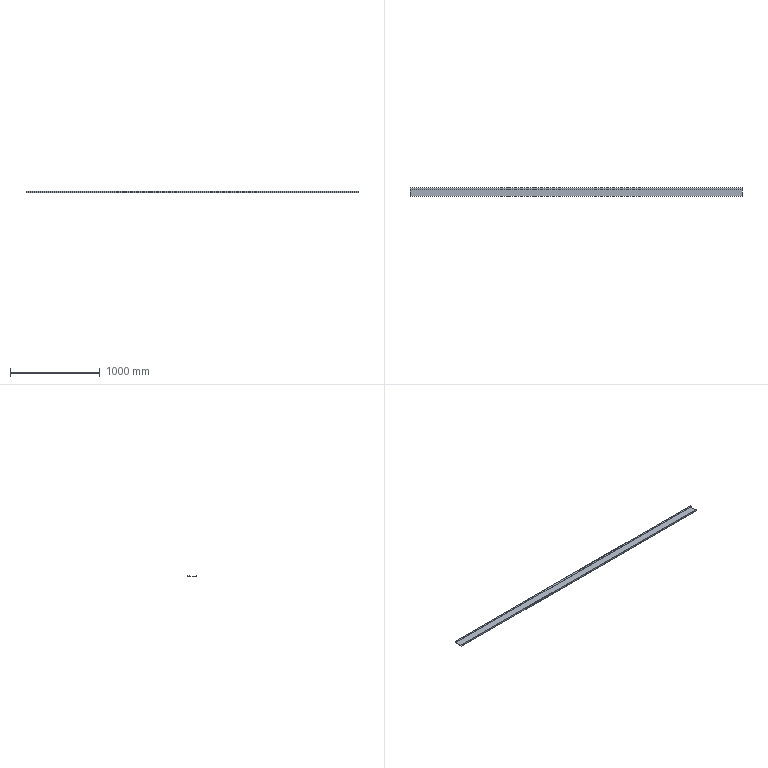Part | STEP file | Powder bin toe plate 3 | 1 solid | 18 faces | box 3694 x 100 x 20 mm | volume 849140 mm3 | plane 12 | cylinder 6 | commonest cylinder face diameters 2 x3 5 x3
STEP:
#1=CARTESIAN_POINT('',(0.,0.,0.));
#2=DIRECTION('',(0.,0.,1.));
#3=DIRECTION('',(1.,0.,0.));
#4=AXIS2_PLACEMENT_3D('',#1,#2,#3);
#5=CARTESIAN_POINT('',(-1847.,1.5,2.5));
#6=VERTEX_POINT('',#5);
#7=CARTESIAN_POINT('',(-1847.,1.5,20.));
#8=VERTEX_POINT('',#7);
#9=CARTESIAN_POINT('',(-1847.,1.5,2.5));
#10=DIRECTION('',(0.,0.,1.));
#11=VECTOR('',#10,1.);
#12=LINE('',#9,#11);
#13=CARTESIAN_POINT('',(1847.,1.5,2.5));
#14=DIRECTION('',(0.,-1.,0.));
#15=DIRECTION('',(0.,0.,-1.));
#16=AXIS2_PLACEMENT_3D('',#13,#14,#15);
#17=PLANE('',#16);
#18=CARTESIAN_POINT('',(0.,-3694.));
#19=DIRECTION('',(-1.,0.));
#20=VECTOR('',#19,1.);
#21=LINE('',#18,#20);
#22=(GEOMETRIC_REPRESENTATION_CONTEXT(2)PARAMETRIC_REPRESENTATION_CONTEXT()REPRESENTATION_CONTEXT('',''));
#23=DEFINITIONAL_REPRESENTATION('',(#21),#22);
#24=PCURVE('',#17,#23);
#25=CARTESIAN_POINT('',(-1847.,2.5,2.5));
#26=DIRECTION('',(-1.,0.,0.));
#27=DIRECTION('',(0.,0.,1.));
#28=AXIS2_PLACEMENT_3D('',#25,#26,#27);
#29=PLANE('',#28);
#30=CARTESIAN_POINT('',(0.,-1.));
#31=DIRECTION('',(1.,0.));
#32=VECTOR('',#31,1.);
#33=LINE('',#30,#32);
#34=(GEOMETRIC_REPRESENTATION_CONTEXT(2)PARAMETRIC_REPRESENTATION_CONTEXT()REPRESENTATION_CONTEXT('',''));
#35=DEFINITIONAL_REPRESENTATION('',(#33),#34);
#36=PCURVE('',#29,#35);
#37=SURFACE_CURVE('',#12,(#24,#36),.PCURVE_S1.);
#38=EDGE_CURVE('',#6,#8,#37,.T.);
#39=ORIENTED_EDGE('',*,*,#38,.T.);
#40=CARTESIAN_POINT('',(1847.,1.5,20.));
#41=VERTEX_POINT('',#40);
#42=CARTESIAN_POINT('',(1847.,1.5,20.));
#43=DIRECTION('',(-1.,0.,0.));
#44=VECTOR('',#43,1.);
#45=LINE('',#42,#44);
#46=CARTESIAN_POINT('',(-17.5,0.));
#47=DIRECTION('',(0.,-1.));
#48=VECTOR('',#47,1.);
#49=LINE('',#46,#48);
#50=(GEOMETRIC_REPRESENTATION_CONTEXT(2)PARAMETRIC_REPRESENTATION_CONTEXT()REPRESENTATION_CONTEXT('',''));
#51=DEFINITIONAL_REPRESENTATION('',(#49),#50);
#52=PCURVE('',#17,#51);
#53=CARTESIAN_POINT('',(1847.,0.,20.));
#54=DIRECTION('',(0.,0.,1.));
#55=DIRECTION('',(1.,0.,0.));
#56=AXIS2_PLACEMENT_3D('',#53,#54,#55);
#57=PLANE('',#56);
#58=CARTESIAN_POINT('',(0.,1.5));
#59=DIRECTION('',(-1.,0.));
#60=VECTOR('',#59,1.);
#61=LINE('',#58,#60);
#62=(GEOMETRIC_REPRESENTATION_CONTEXT(2)PARAMETRIC_REPRESENTATION_CONTEXT()REPRESENTATION_CONTEXT('',''));
#63=DEFINITIONAL_REPRESENTATION('',(#61),#62);
#64=PCURVE('',#57,#63);
#65=SURFACE_CURVE('',#45,(#52,#64),.PCURVE_S1.);
#66=EDGE_CURVE('',#41,#8,#65,.T.);
#67=ORIENTED_EDGE('',*,*,#66,.F.);
#68=CARTESIAN_POINT('',(1847.,1.5,2.5));
#69=VERTEX_POINT('',#68);
#70=CARTESIAN_POINT('',(1847.,1.5,2.5));
#71=DIRECTION('',(0.,0.,1.));
#72=VECTOR('',#71,1.);
#73=LINE('',#70,#72);
#74=CARTESIAN_POINT('',(0.,0.));
#75=DIRECTION('',(-1.,0.));
#76=VECTOR('',#75,1.);
#77=LINE('',#74,#76);
#78=(GEOMETRIC_REPRESENTATION_CONTEXT(2)PARAMETRIC_REPRESENTATION_CONTEXT()REPRESENTATION_CONTEXT('',''));
#79=DEFINITIONAL_REPRESENTATION('',(#77),#78);
#80=PCURVE('',#17,#79);
#81=CARTESIAN_POINT('',(1847.,2.5,2.5));
#82=DIRECTION('',(-1.,0.,0.));
#83=DIRECTION('',(0.,0.,1.));
#84=AXIS2_PLACEMENT_3D('',#81,#82,#83);
#85=PLANE('',#84);
#86=CARTESIAN_POINT('',(0.,-1.));
#87=DIRECTION('',(1.,0.));
#88=VECTOR('',#87,1.);
#89=LINE('',#86,#88);
#90=(GEOMETRIC_REPRESENTATION_CONTEXT(2)PARAMETRIC_REPRESENTATION_CONTEXT()REPRESENTATION_CONTEXT('',''));
#91=DEFINITIONAL_REPRESENTATION('',(#89),#90);
#92=PCURVE('',#85,#91);
#93=SURFACE_CURVE('',#73,(#80,#92),.PCURVE_S1.);
#94=EDGE_CURVE('',#69,#41,#93,.T.);
#95=ORIENTED_EDGE('',*,*,#94,.F.);
#96=CARTESIAN_POINT('',(1847.,1.5,2.5));
#97=DIRECTION('',(-1.,0.,0.));
#98=VECTOR('',#97,1.);
#99=LINE('',#96,#98);
#100=CARTESIAN_POINT('',(0.,0.));
#101=DIRECTION('',(0.,-1.));
#102=VECTOR('',#101,1.);
#103=LINE('',#100,#102);
#104=(GEOMETRIC_REPRESENTATION_CONTEXT(2)PARAMETRIC_REPRESENTATION_CONTEXT()REPRESENTATION_CONTEXT('',''));
#105=DEFINITIONAL_REPRESENTATION('',(#103),#104);
#106=PCURVE('',#17,#105);
#107=CARTESIAN_POINT('',(1847.,2.5,2.5));
#108=DIRECTION('',(-1.,0.,0.));
#109=DIRECTION('',(0.,0.,1.));
#110=AXIS2_PLACEMENT_3D('',#107,#108,#109);
#111=CYLINDRICAL_SURFACE('',#110,1.);
#112=CARTESIAN_POINT('',(4.712,0.));
#113=DIRECTION('',(0.,1.));
#114=VECTOR('',#113,1.);
#115=LINE('',#112,#114);
#116=(GEOMETRIC_REPRESENTATION_CONTEXT(2)PARAMETRIC_REPRESENTATION_CONTEXT()REPRESENTATION_CONTEXT('',''));
#117=DEFINITIONAL_REPRESENTATION('',(#115),#116);
#118=PCURVE('',#111,#117);
#119=SURFACE_CURVE('',#99,(#106,#118),.PCURVE_S1.);
#120=EDGE_CURVE('',#69,#6,#119,.T.);
#121=ORIENTED_EDGE('',*,*,#120,.T.);
#122=EDGE_LOOP('',(#39,#67,#95,#121));
#123=FACE_BOUND('',#122,.T.);
#124=ADVANCED_FACE('',(#123),#17,.F.);
#125=CARTESIAN_POINT('',(-1847.,0.,20.));
#126=VERTEX_POINT('',#125);
#127=CARTESIAN_POINT('',(-1847.,0.,20.));
#128=DIRECTION('',(0.,1.,0.));
#129=VECTOR('',#128,1.);
#130=LINE('',#127,#129);
#131=CARTESIAN_POINT('',(-3694.,0.));
#132=DIRECTION('',(0.,1.));
#133=VECTOR('',#132,1.);
#134=LINE('',#131,#133);
#135=(GEOMETRIC_REPRESENTATION_CONTEXT(2)PARAMETRIC_REPRESENTATION_CONTEXT()REPRESENTATION_CONTEXT('',''));
#136=DEFINITIONAL_REPRESENTATION('',(#134),#135);
#137=PCURVE('',#57,#136);
#138=CARTESIAN_POINT('',(17.5,-2.5));
#139=DIRECTION('',(0.,1.));
#140=VECTOR('',#139,1.);
#141=LINE('',#138,#140);
#142=(GEOMETRIC_REPRESENTATION_CONTEXT(2)PARAMETRIC_REPRESENTATION_CONTEXT()REPRESENTATION_CONTEXT('',''));
#143=DEFINITIONAL_REPRESENTATION('',(#141),#142);
#144=PCURVE('',#29,#143);
#145=SURFACE_CURVE('',#130,(#137,#144),.PCURVE_S1.);
#146=EDGE_CURVE('',#126,#8,#145,.T.);
#147=ORIENTED_EDGE('',*,*,#146,.F.);
#148=CARTESIAN_POINT('',(1847.,0.,20.));
#149=VERTEX_POINT('',#148);
#150=CARTESIAN_POINT('',(1847.,0.,20.));
#151=DIRECTION('',(-1.,0.,0.));
#152=VECTOR('',#151,1.);
#153=LINE('',#150,#152);
#154=CARTESIAN_POINT('',(0.,0.));
#155=DIRECTION('',(-1.,0.));
#156=VECTOR('',#155,1.);
#157=LINE('',#154,#156);
#158=(GEOMETRIC_REPRESENTATION_CONTEXT(2)PARAMETRIC_REPRESENTATION_CONTEXT()REPRESENTATION_CONTEXT('',''));
#159=DEFINITIONAL_REPRESENTATION('',(#157),#158);
#160=PCURVE('',#57,#159);
#161=CARTESIAN_POINT('',(1847.,0.,2.5));
#162=DIRECTION('',(0.,-1.,0.));
#163=DIRECTION('',(0.,0.,-1.));
#164=AXIS2_PLACEMENT_3D('',#161,#162,#163);
#165=PLANE('',#164);
#166=CARTESIAN_POINT('',(-17.5,0.));
#167=DIRECTION('',(0.,-1.));
#168=VECTOR('',#167,1.);
#169=LINE('',#166,#168);
#170=(GEOMETRIC_REPRESENTATION_CONTEXT(2)PARAMETRIC_REPRESENTATION_CONTEXT()REPRESENTATION_CONTEXT('',''));
#171=DEFINITIONAL_REPRESENTATION('',(#169),#170);
#172=PCURVE('',#165,#171);
#173=SURFACE_CURVE('',#153,(#160,#172),.PCURVE_S1.);
#174=EDGE_CURVE('',#149,#126,#173,.T.);
#175=ORIENTED_EDGE('',*,*,#174,.F.);
#176=CARTESIAN_POINT('',(1847.,0.,20.));
#177=DIRECTION('',(0.,1.,0.));
#178=VECTOR('',#177,1.);
#179=LINE('',#176,#178);
#180=CARTESIAN_POINT('',(0.,0.));
#181=DIRECTION('',(0.,1.));
#182=VECTOR('',#181,1.);
#183=LINE('',#180,#182);
#184=(GEOMETRIC_REPRESENTATION_CONTEXT(2)PARAMETRIC_REPRESENTATION_CONTEXT()REPRESENTATION_CONTEXT('',''));
#185=DEFINITIONAL_REPRESENTATION('',(#183),#184);
#186=PCURVE('',#57,#185);
#187=CARTESIAN_POINT('',(17.5,-2.5));
#188=DIRECTION('',(0.,1.));
#189=VECTOR('',#188,1.);
#190=LINE('',#187,#189);
#191=(GEOMETRIC_REPRESENTATION_CONTEXT(2)PARAMETRIC_REPRESENTATION_CONTEXT()REPRESENTATION_CONTEXT('',''));
#192=DEFINITIONAL_REPRESENTATION('',(#190),#191);
#193=PCURVE('',#85,#192);
#194=SURFACE_CURVE('',#179,(#186,#193),.PCURVE_S1.);
#195=EDGE_CURVE('',#149,#41,#194,.T.);
#196=ORIENTED_EDGE('',*,*,#195,.T.);
#197=ORIENTED_EDGE('',*,*,#66,.T.);
#198=EDGE_LOOP('',(#147,#175,#196,#197));
#199=FACE_BOUND('',#198,.T.);
#200=ADVANCED_FACE('',(#199),#57,.T.);
#201=CARTESIAN_POINT('',(-1847.,0.,2.5));
#202=VERTEX_POINT('',#201);
#203=CARTESIAN_POINT('',(-1847.,0.,2.5));
#204=DIRECTION('',(0.,0.,1.));
#205=VECTOR('',#204,1.);
#206=LINE('',#203,#205);
#207=CARTESIAN_POINT('',(0.,-3694.));
#208=DIRECTION('',(-1.,0.));
#209=VECTOR('',#208,1.);
#210=LINE('',#207,#209);
#211=(GEOMETRIC_REPRESENTATION_CONTEXT(2)PARAMETRIC_REPRESENTATION_CONTEXT()REPRESENTATION_CONTEXT('',''));
#212=DEFINITIONAL_REPRESENTATION('',(#210),#211);
#213=PCURVE('',#165,#212);
#214=CARTESIAN_POINT('',(0.,-2.5));
#215=DIRECTION('',(1.,0.));
#216=VECTOR('',#215,1.);
#217=LINE('',#214,#216);
#218=(GEOMETRIC_REPRESENTATION_CONTEXT(2)PARAMETRIC_REPRESENTATION_CONTEXT()REPRESENTATION_CONTEXT('',''));
#219=DEFINITIONAL_REPRESENTATION('',(#217),#218);
#220=PCURVE('',#29,#219);
#221=SURFACE_CURVE('',#206,(#213,#220),.PCURVE_S1.);
#222=EDGE_CURVE('',#202,#126,#221,.T.);
#223=ORIENTED_EDGE('',*,*,#222,.F.);
#224=CARTESIAN_POINT('',(1847.,0.,2.5));
#225=VERTEX_POINT('',#224);
#226=CARTESIAN_POINT('',(1847.,0.,2.5));
#227=DIRECTION('',(-1.,0.,0.));
#228=VECTOR('',#227,1.);
#229=LINE('',#226,#228);
#230=CARTESIAN_POINT('',(0.,0.));
#231=DIRECTION('',(0.,-1.));
#232=VECTOR('',#231,1.);
#233=LINE('',#230,#232);
#234=(GEOMETRIC_REPRESENTATION_CONTEXT(2)PARAMETRIC_REPRESENTATION_CONTEXT()REPRESENTATION_CONTEXT('',''));
#235=DEFINITIONAL_REPRESENTATION('',(#233),#234);
#236=PCURVE('',#165,#235);
#237=CARTESIAN_POINT('',(1847.,2.5,2.5));
#238=DIRECTION('',(-1.,0.,0.));
#239=DIRECTION('',(0.,0.,1.));
#240=AXIS2_PLACEMENT_3D('',#237,#238,#239);
#241=CYLINDRICAL_SURFACE('',#240,2.5);
#242=CARTESIAN_POINT('',(4.712,0.));
#243=DIRECTION('',(0.,1.));
#244=VECTOR('',#243,1.);
#245=LINE('',#242,#244);
#246=(GEOMETRIC_REPRESENTATION_CONTEXT(2)PARAMETRIC_REPRESENTATION_CONTEXT()REPRESENTATION_CONTEXT('',''));
#247=DEFINITIONAL_REPRESENTATION('',(#245),#246);
#248=PCURVE('',#241,#247);
#249=SURFACE_CURVE('',#229,(#236,#248),.PCURVE_S1.);
#250=EDGE_CURVE('',#225,#202,#249,.T.);
#251=ORIENTED_EDGE('',*,*,#250,.F.);
#252=CARTESIAN_POINT('',(1847.,0.,2.5));
#253=DIRECTION('',(0.,0.,1.));
#254=VECTOR('',#253,1.);
#255=LINE('',#252,#254);
#256=CARTESIAN_POINT('',(0.,0.));
#257=DIRECTION('',(-1.,0.));
#258=VECTOR('',#257,1.);
#259=LINE('',#256,#258);
#260=(GEOMETRIC_REPRESENTATION_CONTEXT(2)PARAMETRIC_REPRESENTATION_CONTEXT()REPRESENTATION_CONTEXT('',''));
#261=DEFINITIONAL_REPRESENTATION('',(#259),#260);
#262=PCURVE('',#165,#261);
#263=CARTESIAN_POINT('',(0.,-2.5));
#264=DIRECTION('',(1.,0.));
#265=VECTOR('',#264,1.);
#266=LINE('',#263,#265);
#267=(GEOMETRIC_REPRESENTATION_CONTEXT(2)PARAMETRIC_REPRESENTATION_CONTEXT()REPRESENTATION_CONTEXT('',''));
#268=DEFINITIONAL_REPRESENTATION('',(#266),#267);
#269=PCURVE('',#85,#268);
#270=SURFACE_CURVE('',#255,(#262,#269),.PCURVE_S1.);
#271=EDGE_CURVE('',#225,#149,#270,.T.);
#272=ORIENTED_EDGE('',*,*,#271,.T.);
#273=ORIENTED_EDGE('',*,*,#174,.T.);
#274=EDGE_LOOP('',(#223,#251,#272,#273));
#275=FACE_BOUND('',#274,.T.);
#276=ADVANCED_FACE('',(#275),#165,.T.);
#277=CARTESIAN_POINT('',(-1847.,2.5,0.));
#278=VERTEX_POINT('',#277);
#279=CARTESIAN_POINT('',(-1847.,2.5,2.5));
#280=DIRECTION('',(-1.,0.,0.));
#281=DIRECTION('',(0.,0.,1.));
#282=AXIS2_PLACEMENT_3D('',#279,#280,#281);
#283=CIRCLE('',#282,2.5);
#284=CARTESIAN_POINT('',(0.,3694.));
#285=DIRECTION('',(1.,0.));
#286=VECTOR('',#285,1.);
#287=LINE('',#284,#286);
#288=(GEOMETRIC_REPRESENTATION_CONTEXT(2)PARAMETRIC_REPRESENTATION_CONTEXT()REPRESENTATION_CONTEXT('',''));
#289=DEFINITIONAL_REPRESENTATION('',(#287),#288);
#290=PCURVE('',#241,#289);
#291=CARTESIAN_POINT('',(0.,0.));
#292=DIRECTION('',(1.,0.));
#293=AXIS2_PLACEMENT_2D('',#291,#292);
#294=CIRCLE('',#293,2.5);
#295=(GEOMETRIC_REPRESENTATION_CONTEXT(2)PARAMETRIC_REPRESENTATION_CONTEXT()REPRESENTATION_CONTEXT('',''));
#296=DEFINITIONAL_REPRESENTATION('',(#294),#295);
#297=PCURVE('',#29,#296);
#298=SURFACE_CURVE('',#283,(#290,#297),.PCURVE_S1.);
#299=EDGE_CURVE('',#278,#202,#298,.T.);
#300=ORIENTED_EDGE('',*,*,#299,.F.);
#301=CARTESIAN_POINT('',(1847.,2.5,0.));
#302=VERTEX_POINT('',#301);
#303=CARTESIAN_POINT('',(1847.,2.5,0.));
#304=DIRECTION('',(-1.,0.,0.));
#305=VECTOR('',#304,1.);
#306=LINE('',#303,#305);
#307=CARTESIAN_POINT('',(3.142,0.));
#308=DIRECTION('',(0.,1.));
#309=VECTOR('',#308,1.);
#310=LINE('',#307,#309);
#311=(GEOMETRIC_REPRESENTATION_CONTEXT(2)PARAMETRIC_REPRESENTATION_CONTEXT()REPRESENTATION_CONTEXT('',''));
#312=DEFINITIONAL_REPRESENTATION('',(#310),#311);
#313=PCURVE('',#241,#312);
#314=CARTESIAN_POINT('',(1847.,2.5,0.));
#315=DIRECTION('',(0.,0.,-1.));
#316=DIRECTION('',(-1.,0.,0.));
#317=AXIS2_PLACEMENT_3D('',#314,#315,#316);
#318=PLANE('',#317);
#319=CARTESIAN_POINT('',(0.,0.));
#320=DIRECTION('',(1.,0.));
#321=VECTOR('',#320,1.);
#322=LINE('',#319,#321);
#323=(GEOMETRIC_REPRESENTATION_CONTEXT(2)PARAMETRIC_REPRESENTATION_CONTEXT()REPRESENTATION_CONTEXT('',''));
#324=DEFINITIONAL_REPRESENTATION('',(#322),#323);
#325=PCURVE('',#318,#324);
#326=SURFACE_CURVE('',#306,(#313,#325),.PCURVE_S1.);
#327=EDGE_CURVE('',#302,#278,#326,.T.);
#328=ORIENTED_EDGE('',*,*,#327,.F.);
#329=CARTESIAN_POINT('',(1847.,2.5,2.5));
#330=DIRECTION('',(-1.,0.,0.));
#331=DIRECTION('',(0.,0.,1.));
#332=AXIS2_PLACEMENT_3D('',#329,#330,#331);
#333=CIRCLE('',#332,2.5);
#334=CARTESIAN_POINT('',(0.,0.));
#335=DIRECTION('',(1.,0.));
#336=VECTOR('',#335,1.);
#337=LINE('',#334,#336);
#338=(GEOMETRIC_REPRESENTATION_CONTEXT(2)PARAMETRIC_REPRESENTATION_CONTEXT()REPRESENTATION_CONTEXT('',''));
#339=DEFINITIONAL_REPRESENTATION('',(#337),#338);
#340=PCURVE('',#241,#339);
#341=CARTESIAN_POINT('',(0.,0.));
#342=DIRECTION('',(1.,0.));
#343=AXIS2_PLACEMENT_2D('',#341,#342);
#344=CIRCLE('',#343,2.5);
#345=(GEOMETRIC_REPRESENTATION_CONTEXT(2)PARAMETRIC_REPRESENTATION_CONTEXT()REPRESENTATION_CONTEXT('',''));
#346=DEFINITIONAL_REPRESENTATION('',(#344),#345);
#347=PCURVE('',#85,#346);
#348=SURFACE_CURVE('',#333,(#340,#347),.PCURVE_S1.);
#349=EDGE_CURVE('',#302,#225,#348,.T.);
#350=ORIENTED_EDGE('',*,*,#349,.T.);
#351=ORIENTED_EDGE('',*,*,#250,.T.);
#352=EDGE_LOOP('',(#300,#328,#350,#351));
#353=FACE_BOUND('',#352,.T.);
#354=ADVANCED_FACE('',(#353),#241,.T.);
#355=CARTESIAN_POINT('',(-1847.,97.5,0.));
#356=VERTEX_POINT('',#355);
#357=CARTESIAN_POINT('',(-1847.,2.5,0.));
#358=DIRECTION('',(0.,-1.,0.));
#359=VECTOR('',#358,1.);
#360=LINE('',#357,#359);
#361=CARTESIAN_POINT('',(3694.,0.));
#362=DIRECTION('',(0.,-1.));
#363=VECTOR('',#362,1.);
#364=LINE('',#361,#363);
#365=(GEOMETRIC_REPRESENTATION_CONTEXT(2)PARAMETRIC_REPRESENTATION_CONTEXT()REPRESENTATION_CONTEXT('',''));
#366=DEFINITIONAL_REPRESENTATION('',(#364),#365);
#367=PCURVE('',#318,#366);
#368=CARTESIAN_POINT('',(-2.5,0.));
#369=DIRECTION('',(0.,-1.));
#370=VECTOR('',#369,1.);
#371=LINE('',#368,#370);
#372=(GEOMETRIC_REPRESENTATION_CONTEXT(2)PARAMETRIC_REPRESENTATION_CONTEXT()REPRESENTATION_CONTEXT('',''));
#373=DEFINITIONAL_REPRESENTATION('',(#371),#372);
#374=PCURVE('',#29,#373);
#375=SURFACE_CURVE('',#360,(#367,#374),.PCURVE_S1.);
#376=EDGE_CURVE('',#356,#278,#375,.T.);
#377=ORIENTED_EDGE('',*,*,#376,.F.);
#378=CARTESIAN_POINT('',(1847.,97.5,0.));
#379=VERTEX_POINT('',#378);
#380=CARTESIAN_POINT('',(1847.,97.5,0.));
#381=DIRECTION('',(-1.,0.,0.));
#382=VECTOR('',#381,1.);
#383=LINE('',#380,#382);
#384=CARTESIAN_POINT('',(0.,95.));
#385=DIRECTION('',(1.,0.));
#386=VECTOR('',#385,1.);
#387=LINE('',#384,#386);
#388=(GEOMETRIC_REPRESENTATION_CONTEXT(2)PARAMETRIC_REPRESENTATION_CONTEXT()REPRESENTATION_CONTEXT('',''));
#389=DEFINITIONAL_REPRESENTATION('',(#387),#388);
#390=PCURVE('',#318,#389);
#391=CARTESIAN_POINT('',(1847.,97.5,2.5));
#392=DIRECTION('',(-1.,0.,0.));
#393=DIRECTION('',(0.,0.,1.));
#394=AXIS2_PLACEMENT_3D('',#391,#392,#393);
#395=CYLINDRICAL_SURFACE('',#394,2.5);
#396=CARTESIAN_POINT('',(3.142,0.));
#397=DIRECTION('',(0.,1.));
#398=VECTOR('',#397,1.);
#399=LINE('',#396,#398);
#400=(GEOMETRIC_REPRESENTATION_CONTEXT(2)PARAMETRIC_REPRESENTATION_CONTEXT()REPRESENTATION_CONTEXT('',''));
#401=DEFINITIONAL_REPRESENTATION('',(#399),#400);
#402=PCURVE('',#395,#401);
#403=SURFACE_CURVE('',#383,(#390,#402),.PCURVE_S1.);
#404=EDGE_CURVE('',#379,#356,#403,.T.);
#405=ORIENTED_EDGE('',*,*,#404,.F.);
#406=CARTESIAN_POINT('',(1847.,2.5,0.));
#407=DIRECTION('',(0.,-1.,0.));
#408=VECTOR('',#407,1.);
#409=LINE('',#406,#408);
#410=CARTESIAN_POINT('',(0.,0.));
#411=DIRECTION('',(0.,-1.));
#412=VECTOR('',#411,1.);
#413=LINE('',#410,#412);
#414=(GEOMETRIC_REPRESENTATION_CONTEXT(2)PARAMETRIC_REPRESENTATION_CONTEXT()REPRESENTATION_CONTEXT('',''));
#415=DEFINITIONAL_REPRESENTATION('',(#413),#414);
#416=PCURVE('',#318,#415);
#417=CARTESIAN_POINT('',(-2.5,0.));
#418=DIRECTION('',(0.,-1.));
#419=VECTOR('',#418,1.);
#420=LINE('',#417,#419);
#421=(GEOMETRIC_REPRESENTATION_CONTEXT(2)PARAMETRIC_REPRESENTATION_CONTEXT()REPRESENTATION_CONTEXT('',''));
#422=DEFINITIONAL_REPRESENTATION('',(#420),#421);
#423=PCURVE('',#85,#422);
#424=SURFACE_CURVE('',#409,(#416,#423),.PCURVE_S1.);
#425=EDGE_CURVE('',#379,#302,#424,.T.);
#426=ORIENTED_EDGE('',*,*,#425,.T.);
#427=ORIENTED_EDGE('',*,*,#327,.T.);
#428=EDGE_LOOP('',(#377,#405,#426,#427));
#429=FACE_BOUND('',#428,.T.);
#430=ADVANCED_FACE('',(#429),#318,.T.);
#431=CARTESIAN_POINT('',(-1847.,100.,2.5));
#432=VERTEX_POINT('',#431);
#433=CARTESIAN_POINT('',(-1847.,97.5,2.5));
#434=DIRECTION('',(-1.,0.,0.));
#435=DIRECTION('',(0.,0.,-1.));
#436=AXIS2_PLACEMENT_3D('',#433,#434,#435);
#437=CIRCLE('',#436,2.5);
#438=CARTESIAN_POINT('',(-3.142,3694.));
#439=DIRECTION('',(1.,0.));
#440=VECTOR('',#439,1.);
#441=LINE('',#438,#440);
#442=(GEOMETRIC_REPRESENTATION_CONTEXT(2)PARAMETRIC_REPRESENTATION_CONTEXT()REPRESENTATION_CONTEXT('',''));
#443=DEFINITIONAL_REPRESENTATION('',(#441),#442);
#444=PCURVE('',#395,#443);
#445=CARTESIAN_POINT('',(0.,95.));
#446=DIRECTION('',(-1.,0.));
#447=AXIS2_PLACEMENT_2D('',#445,#446);
#448=CIRCLE('',#447,2.5);
#449=(GEOMETRIC_REPRESENTATION_CONTEXT(2)PARAMETRIC_REPRESENTATION_CONTEXT()REPRESENTATION_CONTEXT('',''));
#450=DEFINITIONAL_REPRESENTATION('',(#448),#449);
#451=PCURVE('',#29,#450);
#452=SURFACE_CURVE('',#437,(#444,#451),.PCURVE_S1.);
#453=EDGE_CURVE('',#432,#356,#452,.T.);
#454=ORIENTED_EDGE('',*,*,#453,.F.);
#455=CARTESIAN_POINT('',(1847.,100.,2.5));
#456=VERTEX_POINT('',#455);
#457=CARTESIAN_POINT('',(1847.,100.,2.5));
#458=DIRECTION('',(-1.,0.,0.));
#459=VECTOR('',#458,1.);
#460=LINE('',#457,#459);
#461=CARTESIAN_POINT('',(1.571,0.));
#462=DIRECTION('',(0.,1.));
#463=VECTOR('',#462,1.);
#464=LINE('',#461,#463);
#465=(GEOMETRIC_REPRESENTATION_CONTEXT(2)PARAMETRIC_REPRESENTATION_CONTEXT()REPRESENTATION_CONTEXT('',''));
#466=DEFINITIONAL_REPRESENTATION('',(#464),#465);
#467=PCURVE('',#395,#466);
#468=CARTESIAN_POINT('',(1847.,100.,2.5));
#469=DIRECTION('',(0.,1.,0.));
#470=DIRECTION('',(0.,0.,1.));
#471=AXIS2_PLACEMENT_3D('',#468,#469,#470);
#472=PLANE('',#471);
#473=CARTESIAN_POINT('',(0.,0.));
#474=DIRECTION('',(0.,-1.));
#475=VECTOR('',#474,1.);
#476=LINE('',#473,#475);
#477=(GEOMETRIC_REPRESENTATION_CONTEXT(2)PARAMETRIC_REPRESENTATION_CONTEXT()REPRESENTATION_CONTEXT('',''));
#478=DEFINITIONAL_REPRESENTATION('',(#476),#477);
#479=PCURVE('',#472,#478);
#480=SURFACE_CURVE('',#460,(#467,#479),.PCURVE_S1.);
#481=EDGE_CURVE('',#456,#432,#480,.T.);
#482=ORIENTED_EDGE('',*,*,#481,.F.);
#483=CARTESIAN_POINT('',(1847.,97.5,2.5));
#484=DIRECTION('',(-1.,0.,0.));
#485=DIRECTION('',(0.,0.,-1.));
#486=AXIS2_PLACEMENT_3D('',#483,#484,#485);
#487=CIRCLE('',#486,2.5);
#488=CARTESIAN_POINT('',(-3.142,0.));
#489=DIRECTION('',(1.,0.));
#490=VECTOR('',#489,1.);
#491=LINE('',#488,#490);
#492=(GEOMETRIC_REPRESENTATION_CONTEXT(2)PARAMETRIC_REPRESENTATION_CONTEXT()REPRESENTATION_CONTEXT('',''));
#493=DEFINITIONAL_REPRESENTATION('',(#491),#492);
#494=PCURVE('',#395,#493);
#495=CARTESIAN_POINT('',(0.,95.));
#496=DIRECTION('',(-1.,0.));
#497=AXIS2_PLACEMENT_2D('',#495,#496);
#498=CIRCLE('',#497,2.5);
#499=(GEOMETRIC_REPRESENTATION_CONTEXT(2)PARAMETRIC_REPRESENTATION_CONTEXT()REPRESENTATION_CONTEXT('',''));
#500=DEFINITIONAL_REPRESENTATION('',(#498),#499);
#501=PCURVE('',#85,#500);
#502=SURFACE_CURVE('',#487,(#494,#501),.PCURVE_S1.);
#503=EDGE_CURVE('',#456,#379,#502,.T.);
#504=ORIENTED_EDGE('',*,*,#503,.T.);
#505=ORIENTED_EDGE('',*,*,#404,.T.);
#506=EDGE_LOOP('',(#454,#482,#504,#505));
#507=FACE_BOUND('',#506,.T.);
#508=ADVANCED_FACE('',(#507),#395,.T.);
#509=CARTESIAN_POINT('',(-1847.,100.,17.5));
#510=VERTEX_POINT('',#509);
#511=CARTESIAN_POINT('',(-1847.,100.,2.5));
#512=DIRECTION('',(0.,0.,-1.));
#513=VECTOR('',#512,1.);
#514=LINE('',#511,#513);
#515=CARTESIAN_POINT('',(0.,-3694.));
#516=DIRECTION('',(-1.,0.));
#517=VECTOR('',#516,1.);
#518=LINE('',#515,#517);
#519=(GEOMETRIC_REPRESENTATION_CONTEXT(2)PARAMETRIC_REPRESENTATION_CONTEXT()REPRESENTATION_CONTEXT('',''));
#520=DEFINITIONAL_REPRESENTATION('',(#518),#519);
#521=PCURVE('',#472,#520);
#522=CARTESIAN_POINT('',(0.,97.5));
#523=DIRECTION('',(-1.,0.));
#524=VECTOR('',#523,1.);
#525=LINE('',#522,#524);
#526=(GEOMETRIC_REPRESENTATION_CONTEXT(2)PARAMETRIC_REPRESENTATION_CONTEXT()REPRESENTATION_CONTEXT('',''));
#527=DEFINITIONAL_REPRESENTATION('',(#525),#526);
#528=PCURVE('',#29,#527);
#529=SURFACE_CURVE('',#514,(#521,#528),.PCURVE_S1.);
#530=EDGE_CURVE('',#510,#432,#529,.T.);
#531=ORIENTED_EDGE('',*,*,#530,.F.);
#532=CARTESIAN_POINT('',(1847.,100.,17.5));
#533=VERTEX_POINT('',#532);
#534=CARTESIAN_POINT('',(1847.,100.,17.5));
#535=DIRECTION('',(-1.,0.,0.));
#536=VECTOR('',#535,1.);
#537=LINE('',#534,#536);
#538=CARTESIAN_POINT('',(15.,0.));
#539=DIRECTION('',(0.,-1.));
#540=VECTOR('',#539,1.);
#541=LINE('',#538,#540);
#542=(GEOMETRIC_REPRESENTATION_CONTEXT(2)PARAMETRIC_REPRESENTATION_CONTEXT()REPRESENTATION_CONTEXT('',''));
#543=DEFINITIONAL_REPRESENTATION('',(#541),#542);
#544=PCURVE('',#472,#543);
#545=CARTESIAN_POINT('',(1847.,97.5,17.5));
#546=DIRECTION('',(-1.,0.,0.));
#547=DIRECTION('',(0.,0.,1.));
#548=AXIS2_PLACEMENT_3D('',#545,#546,#547);
#549=CYLINDRICAL_SURFACE('',#548,2.5);
#550=CARTESIAN_POINT('',(1.571,0.));
#551=DIRECTION('',(0.,1.));
#552=VECTOR('',#551,1.);
#553=LINE('',#550,#552);
#554=(GEOMETRIC_REPRESENTATION_CONTEXT(2)PARAMETRIC_REPRESENTATION_CONTEXT()REPRESENTATION_CONTEXT('',''));
#555=DEFINITIONAL_REPRESENTATION('',(#553),#554);
#556=PCURVE('',#549,#555);
#557=SURFACE_CURVE('',#537,(#544,#556),.PCURVE_S1.);
#558=EDGE_CURVE('',#533,#510,#557,.T.);
#559=ORIENTED_EDGE('',*,*,#558,.F.);
#560=CARTESIAN_POINT('',(1847.,100.,2.5));
#561=DIRECTION('',(0.,0.,-1.));
#562=VECTOR('',#561,1.);
#563=LINE('',#560,#562);
#564=CARTESIAN_POINT('',(0.,0.));
#565=DIRECTION('',(-1.,0.));
#566=VECTOR('',#565,1.);
#567=LINE('',#564,#566);
#568=(GEOMETRIC_REPRESENTATION_CONTEXT(2)PARAMETRIC_REPRESENTATION_CONTEXT()REPRESENTATION_CONTEXT('',''));
#569=DEFINITIONAL_REPRESENTATION('',(#567),#568);
#570=PCURVE('',#472,#569);
#571=CARTESIAN_POINT('',(0.,97.5));
#572=DIRECTION('',(-1.,0.));
#573=VECTOR('',#572,1.);
#574=LINE('',#571,#573);
#575=(GEOMETRIC_REPRESENTATION_CONTEXT(2)PARAMETRIC_REPRESENTATION_CONTEXT()REPRESENTATION_CONTEXT('',''));
#576=DEFINITIONAL_REPRESENTATION('',(#574),#575);
#577=PCURVE('',#85,#576);
#578=SURFACE_CURVE('',#563,(#570,#577),.PCURVE_S1.);
#579=EDGE_CURVE('',#533,#456,#578,.T.);
#580=ORIENTED_EDGE('',*,*,#579,.T.);
#581=ORIENTED_EDGE('',*,*,#481,.T.);
#582=EDGE_LOOP('',(#531,#559,#580,#581));
#583=FACE_BOUND('',#582,.T.);
#584=ADVANCED_FACE('',(#583),#472,.T.);
#585=CARTESIAN_POINT('',(-1847.,97.5,20.));
#586=VERTEX_POINT('',#585);
#587=CARTESIAN_POINT('',(-1847.,97.5,17.5));
#588=DIRECTION('',(-1.,0.,0.));
#589=DIRECTION('',(0.,0.,-1.));
#590=AXIS2_PLACEMENT_3D('',#587,#588,#589);
#591=CIRCLE('',#590,2.5);
#592=CARTESIAN_POINT('',(-3.142,3694.));
#593=DIRECTION('',(1.,0.));
#594=VECTOR('',#593,1.);
#595=LINE('',#592,#594);
#596=(GEOMETRIC_REPRESENTATION_CONTEXT(2)PARAMETRIC_REPRESENTATION_CONTEXT()REPRESENTATION_CONTEXT('',''));
#597=DEFINITIONAL_REPRESENTATION('',(#595),#596);
#598=PCURVE('',#549,#597);
#599=CARTESIAN_POINT('',(15.,95.));
#600=DIRECTION('',(-1.,0.));
#601=AXIS2_PLACEMENT_2D('',#599,#600);
#602=CIRCLE('',#601,2.5);
#603=(GEOMETRIC_REPRESENTATION_CONTEXT(2)PARAMETRIC_REPRESENTATION_CONTEXT()REPRESENTATION_CONTEXT('',''));
#604=DEFINITIONAL_REPRESENTATION('',(#602),#603);
#605=PCURVE('',#29,#604);
#606=SURFACE_CURVE('',#591,(#598,#605),.PCURVE_S1.);
#607=EDGE_CURVE('',#586,#510,#606,.T.);
#608=ORIENTED_EDGE('',*,*,#607,.F.);
#609=CARTESIAN_POINT('',(1847.,97.5,20.));
#610=VERTEX_POINT('',#609);
#611=CARTESIAN_POINT('',(1847.,97.5,20.));
#612=DIRECTION('',(-1.,0.,0.));
#613=VECTOR('',#612,1.);
#614=LINE('',#611,#613);
#615=CARTESIAN_POINT('',(0.,0.));
#616=DIRECTION('',(0.,1.));
#617=VECTOR('',#616,1.);
#618=LINE('',#615,#617);
#619=(GEOMETRIC_REPRESENTATION_CONTEXT(2)PARAMETRIC_REPRESENTATION_CONTEXT()REPRESENTATION_CONTEXT('',''));
#620=DEFINITIONAL_REPRESENTATION('',(#618),#619);
#621=PCURVE('',#549,#620);
#622=CARTESIAN_POINT('',(1847.,97.5,20.));
#623=DIRECTION('',(0.,0.,1.));
#624=DIRECTION('',(1.,0.,0.));
#625=AXIS2_PLACEMENT_3D('',#622,#623,#624);
#626=PLANE('',#625);
#627=CARTESIAN_POINT('',(0.,0.));
#628=DIRECTION('',(-1.,0.));
#629=VECTOR('',#628,1.);
#630=LINE('',#627,#629);
#631=(GEOMETRIC_REPRESENTATION_CONTEXT(2)PARAMETRIC_REPRESENTATION_CONTEXT()REPRESENTATION_CONTEXT('',''));
#632=DEFINITIONAL_REPRESENTATION('',(#630),#631);
#633=PCURVE('',#626,#632);
#634=SURFACE_CURVE('',#614,(#621,#633),.PCURVE_S1.);
#635=EDGE_CURVE('',#610,#586,#634,.T.);
#636=ORIENTED_EDGE('',*,*,#635,.F.);
#637=CARTESIAN_POINT('',(1847.,97.5,17.5));
#638=DIRECTION('',(-1.,0.,0.));
#639=DIRECTION('',(0.,0.,-1.));
#640=AXIS2_PLACEMENT_3D('',#637,#638,#639);
#641=CIRCLE('',#640,2.5);
#642=CARTESIAN_POINT('',(-3.142,0.));
#643=DIRECTION('',(1.,0.));
#644=VECTOR('',#643,1.);
#645=LINE('',#642,#644);
#646=(GEOMETRIC_REPRESENTATION_CONTEXT(2)PARAMETRIC_REPRESENTATION_CONTEXT()REPRESENTATION_CONTEXT('',''));
#647=DEFINITIONAL_REPRESENTATION('',(#645),#646);
#648=PCURVE('',#549,#647);
#649=CARTESIAN_POINT('',(15.,95.));
#650=DIRECTION('',(-1.,0.));
#651=AXIS2_PLACEMENT_2D('',#649,#650);
#652=CIRCLE('',#651,2.5);
#653=(GEOMETRIC_REPRESENTATION_CONTEXT(2)PARAMETRIC_REPRESENTATION_CONTEXT()REPRESENTATION_CONTEXT('',''));
#654=DEFINITIONAL_REPRESENTATION('',(#652),#653);
#655=PCURVE('',#85,#654);
#656=SURFACE_CURVE('',#641,(#648,#655),.PCURVE_S1.);
#657=EDGE_CURVE('',#610,#533,#656,.T.);
#658=ORIENTED_EDGE('',*,*,#657,.T.);
#659=ORIENTED_EDGE('',*,*,#558,.T.);
#660=EDGE_LOOP('',(#608,#636,#658,#659));
#661=FACE_BOUND('',#660,.T.);
#662=ADVANCED_FACE('',(#661),#549,.T.);
#663=CARTESIAN_POINT('',(-1847.,80.,20.));
#664=VERTEX_POINT('',#663);
#665=CARTESIAN_POINT('',(-1847.,97.5,20.));
#666=DIRECTION('',(0.,1.,0.));
#667=VECTOR('',#666,1.);
#668=LINE('',#665,#667);
#669=CARTESIAN_POINT('',(-3694.,0.));
#670=DIRECTION('',(0.,1.));
#671=VECTOR('',#670,1.);
#672=LINE('',#669,#671);
#673=(GEOMETRIC_REPRESENTATION_CONTEXT(2)PARAMETRIC_REPRESENTATION_CONTEXT()REPRESENTATION_CONTEXT('',''));
#674=DEFINITIONAL_REPRESENTATION('',(#672),#673);
#675=PCURVE('',#626,#674);
#676=CARTESIAN_POINT('',(17.5,95.));
#677=DIRECTION('',(0.,1.));
#678=VECTOR('',#677,1.);
#679=LINE('',#676,#678);
#680=(GEOMETRIC_REPRESENTATION_CONTEXT(2)PARAMETRIC_REPRESENTATION_CONTEXT()REPRESENTATION_CONTEXT('',''));
#681=DEFINITIONAL_REPRESENTATION('',(#679),#680);
#682=PCURVE('',#29,#681);
#683=SURFACE_CURVE('',#668,(#675,#682),.PCURVE_S1.);
#684=EDGE_CURVE('',#664,#586,#683,.T.);
#685=ORIENTED_EDGE('',*,*,#684,.F.);
#686=CARTESIAN_POINT('',(1847.,80.,20.));
#687=VERTEX_POINT('',#686);
#688=CARTESIAN_POINT('',(1847.,80.,20.));
#689=DIRECTION('',(-1.,0.,0.));
#690=VECTOR('',#689,1.);
#691=LINE('',#688,#690);
#692=CARTESIAN_POINT('',(0.,-17.5));
#693=DIRECTION('',(-1.,0.));
#694=VECTOR('',#693,1.);
#695=LINE('',#692,#694);
#696=(GEOMETRIC_REPRESENTATION_CONTEXT(2)PARAMETRIC_REPRESENTATION_CONTEXT()REPRESENTATION_CONTEXT('',''));
#697=DEFINITIONAL_REPRESENTATION('',(#695),#696);
#698=PCURVE('',#626,#697);
#699=CARTESIAN_POINT('',(1847.,80.,18.5));
#700=DIRECTION('',(0.,-1.,0.));
#701=DIRECTION('',(0.,0.,-1.));
#702=AXIS2_PLACEMENT_3D('',#699,#700,#701);
#703=PLANE('',#702);
#704=CARTESIAN_POINT('',(-1.5,0.));
#705=DIRECTION('',(0.,-1.));
#706=VECTOR('',#705,1.);
#707=LINE('',#704,#706);
#708=(GEOMETRIC_REPRESENTATION_CONTEXT(2)PARAMETRIC_REPRESENTATION_CONTEXT()REPRESENTATION_CONTEXT('',''));
#709=DEFINITIONAL_REPRESENTATION('',(#707),#708);
#710=PCURVE('',#703,#709);
#711=SURFACE_CURVE('',#691,(#698,#710),.PCURVE_S1.);
#712=EDGE_CURVE('',#687,#664,#711,.T.);
#713=ORIENTED_EDGE('',*,*,#712,.F.);
#714=CARTESIAN_POINT('',(1847.,97.5,20.));
#715=DIRECTION('',(0.,1.,0.));
#716=VECTOR('',#715,1.);
#717=LINE('',#714,#716);
#718=CARTESIAN_POINT('',(0.,0.));
#719=DIRECTION('',(0.,1.));
#720=VECTOR('',#719,1.);
#721=LINE('',#718,#720);
#722=(GEOMETRIC_REPRESENTATION_CONTEXT(2)PARAMETRIC_REPRESENTATION_CONTEXT()REPRESENTATION_CONTEXT('',''));
#723=DEFINITIONAL_REPRESENTATION('',(#721),#722);
#724=PCURVE('',#626,#723);
#725=CARTESIAN_POINT('',(17.5,95.));
#726=DIRECTION('',(0.,1.));
#727=VECTOR('',#726,1.);
#728=LINE('',#725,#727);
#729=(GEOMETRIC_REPRESENTATION_CONTEXT(2)PARAMETRIC_REPRESENTATION_CONTEXT()REPRESENTATION_CONTEXT('',''));
#730=DEFINITIONAL_REPRESENTATION('',(#728),#729);
#731=PCURVE('',#85,#730);
#732=SURFACE_CURVE('',#717,(#724,#731),.PCURVE_S1.);
#733=EDGE_CURVE('',#687,#610,#732,.T.);
#734=ORIENTED_EDGE('',*,*,#733,.T.);
#735=ORIENTED_EDGE('',*,*,#635,.T.);
#736=EDGE_LOOP('',(#685,#713,#734,#735));
#737=FACE_BOUND('',#736,.T.);
#738=ADVANCED_FACE('',(#737),#626,.T.);
#739=CARTESIAN_POINT('',(-1847.,80.,18.5));
#740=VERTEX_POINT('',#739);
#741=CARTESIAN_POINT('',(-1847.,80.,18.5));
#742=DIRECTION('',(0.,0.,1.));
#743=VECTOR('',#742,1.);
#744=LINE('',#741,#743);
#745=CARTESIAN_POINT('',(0.,-3694.));
#746=DIRECTION('',(-1.,0.));
#747=VECTOR('',#746,1.);
#748=LINE('',#745,#747);
#749=(GEOMETRIC_REPRESENTATION_CONTEXT(2)PARAMETRIC_REPRESENTATION_CONTEXT()REPRESENTATION_CONTEXT('',''));
#750=DEFINITIONAL_REPRESENTATION('',(#748),#749);
#751=PCURVE('',#703,#750);
#752=CARTESIAN_POINT('',(16.,77.5));
#753=DIRECTION('',(1.,0.));
#754=VECTOR('',#753,1.);
#755=LINE('',#752,#754);
#756=(GEOMETRIC_REPRESENTATION_CONTEXT(2)PARAMETRIC_REPRESENTATION_CONTEXT()REPRESENTATION_CONTEXT('',''));
#757=DEFINITIONAL_REPRESENTATION('',(#755),#756);
#758=PCURVE('',#29,#757);
#759=SURFACE_CURVE('',#744,(#751,#758),.PCURVE_S1.);
#760=EDGE_CURVE('',#740,#664,#759,.T.);
#761=ORIENTED_EDGE('',*,*,#760,.F.);
#762=CARTESIAN_POINT('',(1847.,80.,18.5));
#763=VERTEX_POINT('',#762);
#764=CARTESIAN_POINT('',(1847.,80.,18.5));
#765=DIRECTION('',(-1.,0.,0.));
#766=VECTOR('',#765,1.);
#767=LINE('',#764,#766);
#768=CARTESIAN_POINT('',(0.,0.));
#769=DIRECTION('',(0.,-1.));
#770=VECTOR('',#769,1.);
#771=LINE('',#768,#770);
#772=(GEOMETRIC_REPRESENTATION_CONTEXT(2)PARAMETRIC_REPRESENTATION_CONTEXT()REPRESENTATION_CONTEXT('',''));
#773=DEFINITIONAL_REPRESENTATION('',(#771),#772);
#774=PCURVE('',#703,#773);
#775=CARTESIAN_POINT('',(1847.,97.5,18.5));
#776=DIRECTION('',(0.,0.,1.));
#777=DIRECTION('',(1.,0.,0.));
#778=AXIS2_PLACEMENT_3D('',#775,#776,#777);
#779=PLANE('',#778);
#780=CARTESIAN_POINT('',(0.,-17.5));
#781=DIRECTION('',(-1.,0.));
#782=VECTOR('',#781,1.);
#783=LINE('',#780,#782);
#784=(GEOMETRIC_REPRESENTATION_CONTEXT(2)PARAMETRIC_REPRESENTATION_CONTEXT()REPRESENTATION_CONTEXT('',''));
#785=DEFINITIONAL_REPRESENTATION('',(#783),#784);
#786=PCURVE('',#779,#785);
#787=SURFACE_CURVE('',#767,(#774,#786),.PCURVE_S1.);
#788=EDGE_CURVE('',#763,#740,#787,.T.);
#789=ORIENTED_EDGE('',*,*,#788,.F.);
#790=CARTESIAN_POINT('',(1847.,80.,18.5));
#791=DIRECTION('',(0.,0.,1.));
#792=VECTOR('',#791,1.);
#793=LINE('',#790,#792);
#794=CARTESIAN_POINT('',(0.,0.));
#795=DIRECTION('',(-1.,0.));
#796=VECTOR('',#795,1.);
#797=LINE('',#794,#796);
#798=(GEOMETRIC_REPRESENTATION_CONTEXT(2)PARAMETRIC_REPRESENTATION_CONTEXT()REPRESENTATION_CONTEXT('',''));
#799=DEFINITIONAL_REPRESENTATION('',(#797),#798);
#800=PCURVE('',#703,#799);
#801=CARTESIAN_POINT('',(16.,77.5));
#802=DIRECTION('',(1.,0.));
#803=VECTOR('',#802,1.);
#804=LINE('',#801,#803);
#805=(GEOMETRIC_REPRESENTATION_CONTEXT(2)PARAMETRIC_REPRESENTATION_CONTEXT()REPRESENTATION_CONTEXT('',''));
#806=DEFINITIONAL_REPRESENTATION('',(#804),#805);
#807=PCURVE('',#85,#806);
#808=SURFACE_CURVE('',#793,(#800,#807),.PCURVE_S1.);
#809=EDGE_CURVE('',#763,#687,#808,.T.);
#810=ORIENTED_EDGE('',*,*,#809,.T.);
#811=ORIENTED_EDGE('',*,*,#712,.T.);
#812=EDGE_LOOP('',(#761,#789,#810,#811));
#813=FACE_BOUND('',#812,.T.);
#814=ADVANCED_FACE('',(#813),#703,.T.);
#815=CARTESIAN_POINT('',(-1847.,97.5,18.5));
#816=VERTEX_POINT('',#815);
#817=CARTESIAN_POINT('',(-1847.,97.5,18.5));
#818=DIRECTION('',(0.,1.,0.));
#819=VECTOR('',#818,1.);
#820=LINE('',#817,#819);
#821=CARTESIAN_POINT('',(-3694.,0.));
#822=DIRECTION('',(0.,1.));
#823=VECTOR('',#822,1.);
#824=LINE('',#821,#823);
#825=(GEOMETRIC_REPRESENTATION_CONTEXT(2)PARAMETRIC_REPRESENTATION_CONTEXT()REPRESENTATION_CONTEXT('',''));
#826=DEFINITIONAL_REPRESENTATION('',(#824),#825);
#827=PCURVE('',#779,#826);
#828=CARTESIAN_POINT('',(16.,95.));
#829=DIRECTION('',(0.,1.));
#830=VECTOR('',#829,1.);
#831=LINE('',#828,#830);
#832=(GEOMETRIC_REPRESENTATION_CONTEXT(2)PARAMETRIC_REPRESENTATION_CONTEXT()REPRESENTATION_CONTEXT('',''));
#833=DEFINITIONAL_REPRESENTATION('',(#831),#832);
#834=PCURVE('',#29,#833);
#835=SURFACE_CURVE('',#820,(#827,#834),.PCURVE_S1.);
#836=EDGE_CURVE('',#740,#816,#835,.T.);
#837=ORIENTED_EDGE('',*,*,#836,.T.);
#838=CARTESIAN_POINT('',(1847.,97.5,18.5));
#839=VERTEX_POINT('',#838);
#840=CARTESIAN_POINT('',(1847.,97.5,18.5));
#841=DIRECTION('',(-1.,0.,0.));
#842=VECTOR('',#841,1.);
#843=LINE('',#840,#842);
#844=CARTESIAN_POINT('',(0.,0.));
#845=DIRECTION('',(-1.,0.));
#846=VECTOR('',#845,1.);
#847=LINE('',#844,#846);
#848=(GEOMETRIC_REPRESENTATION_CONTEXT(2)PARAMETRIC_REPRESENTATION_CONTEXT()REPRESENTATION_CONTEXT('',''));
#849=DEFINITIONAL_REPRESENTATION('',(#847),#848);
#850=PCURVE('',#779,#849);
#851=CARTESIAN_POINT('',(1847.,97.5,17.5));
#852=DIRECTION('',(-1.,0.,0.));
#853=DIRECTION('',(0.,0.,1.));
#854=AXIS2_PLACEMENT_3D('',#851,#852,#853);
#855=CYLINDRICAL_SURFACE('',#854,1.);
#856=CARTESIAN_POINT('',(0.,0.));
#857=DIRECTION('',(0.,1.));
#858=VECTOR('',#857,1.);
#859=LINE('',#856,#858);
#860=(GEOMETRIC_REPRESENTATION_CONTEXT(2)PARAMETRIC_REPRESENTATION_CONTEXT()REPRESENTATION_CONTEXT('',''));
#861=DEFINITIONAL_REPRESENTATION('',(#859),#860);
#862=PCURVE('',#855,#861);
#863=SURFACE_CURVE('',#843,(#850,#862),.PCURVE_S1.);
#864=EDGE_CURVE('',#839,#816,#863,.T.);
#865=ORIENTED_EDGE('',*,*,#864,.F.);
#866=CARTESIAN_POINT('',(1847.,97.5,18.5));
#867=DIRECTION('',(0.,1.,0.));
#868=VECTOR('',#867,1.);
#869=LINE('',#866,#868);
#870=CARTESIAN_POINT('',(0.,0.));
#871=DIRECTION('',(0.,1.));
#872=VECTOR('',#871,1.);
#873=LINE('',#870,#872);
#874=(GEOMETRIC_REPRESENTATION_CONTEXT(2)PARAMETRIC_REPRESENTATION_CONTEXT()REPRESENTATION_CONTEXT('',''));
#875=DEFINITIONAL_REPRESENTATION('',(#873),#874);
#876=PCURVE('',#779,#875);
#877=CARTESIAN_POINT('',(16.,95.));
#878=DIRECTION('',(0.,1.));
#879=VECTOR('',#878,1.);
#880=LINE('',#877,#879);
#881=(GEOMETRIC_REPRESENTATION_CONTEXT(2)PARAMETRIC_REPRESENTATION_CONTEXT()REPRESENTATION_CONTEXT('',''));
#882=DEFINITIONAL_REPRESENTATION('',(#880),#881);
#883=PCURVE('',#85,#882);
#884=SURFACE_CURVE('',#869,(#876,#883),.PCURVE_S1.);
#885=EDGE_CURVE('',#763,#839,#884,.T.);
#886=ORIENTED_EDGE('',*,*,#885,.F.);
#887=ORIENTED_EDGE('',*,*,#788,.T.);
#888=EDGE_LOOP('',(#837,#865,#886,#887));
#889=FACE_BOUND('',#888,.T.);
#890=ADVANCED_FACE('',(#889),#779,.F.);
#891=ORIENTED_EDGE('',*,*,#864,.F.);
#892=CARTESIAN_POINT('',(1847.,98.5,17.5));
#893=VERTEX_POINT('',#892);
#894=CARTESIAN_POINT('',(1847.,97.5,17.5));
#895=DIRECTION('',(-1.,0.,0.));
#896=DIRECTION('',(0.,0.,-1.));
#897=AXIS2_PLACEMENT_3D('',#894,#895,#896);
#898=CIRCLE('',#897,1.);
#899=CARTESIAN_POINT('',(-3.142,0.));
#900=DIRECTION('',(1.,0.));
#901=VECTOR('',#900,1.);
#902=LINE('',#899,#901);
#903=(GEOMETRIC_REPRESENTATION_CONTEXT(2)PARAMETRIC_REPRESENTATION_CONTEXT()REPRESENTATION_CONTEXT('',''));
#904=DEFINITIONAL_REPRESENTATION('',(#902),#903);
#905=PCURVE('',#855,#904);
#906=CARTESIAN_POINT('',(15.,95.));
#907=DIRECTION('',(-1.,0.));
#908=AXIS2_PLACEMENT_2D('',#906,#907);
#909=CIRCLE('',#908,1.);
#910=(GEOMETRIC_REPRESENTATION_CONTEXT(2)PARAMETRIC_REPRESENTATION_CONTEXT()REPRESENTATION_CONTEXT('',''));
#911=DEFINITIONAL_REPRESENTATION('',(#909),#910);
#912=PCURVE('',#85,#911);
#913=SURFACE_CURVE('',#898,(#905,#912),.PCURVE_S1.);
#914=EDGE_CURVE('',#839,#893,#913,.T.);
#915=ORIENTED_EDGE('',*,*,#914,.T.);
#916=CARTESIAN_POINT('',(-1847.,98.5,17.5));
#917=VERTEX_POINT('',#916);
#918=CARTESIAN_POINT('',(1847.,98.5,17.5));
#919=DIRECTION('',(-1.,0.,0.));
#920=VECTOR('',#919,1.);
#921=LINE('',#918,#920);
#922=CARTESIAN_POINT('',(1.571,0.));
#923=DIRECTION('',(0.,1.));
#924=VECTOR('',#923,1.);
#925=LINE('',#922,#924);
#926=(GEOMETRIC_REPRESENTATION_CONTEXT(2)PARAMETRIC_REPRESENTATION_CONTEXT()REPRESENTATION_CONTEXT('',''));
#927=DEFINITIONAL_REPRESENTATION('',(#925),#926);
#928=PCURVE('',#855,#927);
#929=CARTESIAN_POINT('',(1847.,98.5,2.5));
#930=DIRECTION('',(0.,1.,0.));
#931=DIRECTION('',(0.,0.,1.));
#932=AXIS2_PLACEMENT_3D('',#929,#930,#931);
#933=PLANE('',#932);
#934=CARTESIAN_POINT('',(15.,0.));
#935=DIRECTION('',(0.,-1.));
#936=VECTOR('',#935,1.);
#937=LINE('',#934,#936);
#938=(GEOMETRIC_REPRESENTATION_CONTEXT(2)PARAMETRIC_REPRESENTATION_CONTEXT()REPRESENTATION_CONTEXT('',''));
#939=DEFINITIONAL_REPRESENTATION('',(#937),#938);
#940=PCURVE('',#933,#939);
#941=SURFACE_CURVE('',#921,(#928,#940),.PCURVE_S1.);
#942=EDGE_CURVE('',#893,#917,#941,.T.);
#943=ORIENTED_EDGE('',*,*,#942,.T.);
#944=CARTESIAN_POINT('',(-1847.,97.5,17.5));
#945=DIRECTION('',(-1.,0.,0.));
#946=DIRECTION('',(0.,0.,-1.));
#947=AXIS2_PLACEMENT_3D('',#944,#945,#946);
#948=CIRCLE('',#947,1.);
#949=CARTESIAN_POINT('',(-3.142,3694.));
#950=DIRECTION('',(1.,0.));
#951=VECTOR('',#950,1.);
#952=LINE('',#949,#951);
#953=(GEOMETRIC_REPRESENTATION_CONTEXT(2)PARAMETRIC_REPRESENTATION_CONTEXT()REPRESENTATION_CONTEXT('',''));
#954=DEFINITIONAL_REPRESENTATION('',(#952),#953);
#955=PCURVE('',#855,#954);
#956=CARTESIAN_POINT('',(15.,95.));
#957=DIRECTION('',(-1.,0.));
#958=AXIS2_PLACEMENT_2D('',#956,#957);
#959=CIRCLE('',#958,1.);
#960=(GEOMETRIC_REPRESENTATION_CONTEXT(2)PARAMETRIC_REPRESENTATION_CONTEXT()REPRESENTATION_CONTEXT('',''));
#961=DEFINITIONAL_REPRESENTATION('',(#959),#960);
#962=PCURVE('',#29,#961);
#963=SURFACE_CURVE('',#948,(#955,#962),.PCURVE_S1.);
#964=EDGE_CURVE('',#816,#917,#963,.T.);
#965=ORIENTED_EDGE('',*,*,#964,.F.);
#966=EDGE_LOOP('',(#891,#915,#943,#965));
#967=FACE_BOUND('',#966,.F.);
#968=ADVANCED_FACE('',(#967),#855,.F.);
#969=CARTESIAN_POINT('',(-1847.,98.5,2.5));
#970=VERTEX_POINT('',#969);
#971=CARTESIAN_POINT('',(-1847.,98.5,2.5));
#972=DIRECTION('',(0.,0.,-1.));
#973=VECTOR('',#972,1.);
#974=LINE('',#971,#973);
#975=CARTESIAN_POINT('',(0.,-3694.));
#976=DIRECTION('',(-1.,0.));
#977=VECTOR('',#976,1.);
#978=LINE('',#975,#977);
#979=(GEOMETRIC_REPRESENTATION_CONTEXT(2)PARAMETRIC_REPRESENTATION_CONTEXT()REPRESENTATION_CONTEXT('',''));
#980=DEFINITIONAL_REPRESENTATION('',(#978),#979);
#981=PCURVE('',#933,#980);
#982=CARTESIAN_POINT('',(0.,96.));
#983=DIRECTION('',(-1.,0.));
#984=VECTOR('',#983,1.);
#985=LINE('',#982,#984);
#986=(GEOMETRIC_REPRESENTATION_CONTEXT(2)PARAMETRIC_REPRESENTATION_CONTEXT()REPRESENTATION_CONTEXT('',''));
#987=DEFINITIONAL_REPRESENTATION('',(#985),#986);
#988=PCURVE('',#29,#987);
#989=SURFACE_CURVE('',#974,(#981,#988),.PCURVE_S1.);
#990=EDGE_CURVE('',#917,#970,#989,.T.);
#991=ORIENTED_EDGE('',*,*,#990,.T.);
#992=CARTESIAN_POINT('',(1847.,98.5,2.5));
#993=VERTEX_POINT('',#992);
#994=CARTESIAN_POINT('',(1847.,98.5,2.5));
#995=DIRECTION('',(-1.,0.,0.));
#996=VECTOR('',#995,1.);
#997=LINE('',#994,#996);
#998=CARTESIAN_POINT('',(0.,0.));
#999=DIRECTION('',(0.,-1.));
#1000=VECTOR('',#999,1.);
#1001=LINE('',#998,#1000);
#1002=(GEOMETRIC_REPRESENTATION_CONTEXT(2)PARAMETRIC_REPRESENTATION_CONTEXT()REPRESENTATION_CONTEXT('',''));
#1003=DEFINITIONAL_REPRESENTATION('',(#1001),#1002);
#1004=PCURVE('',#933,#1003);
#1005=CARTESIAN_POINT('',(1847.,97.5,2.5));
#1006=DIRECTION('',(-1.,0.,0.));
#1007=DIRECTION('',(0.,0.,1.));
#1008=AXIS2_PLACEMENT_3D('',#1005,#1006,#1007);
#1009=CYLINDRICAL_SURFACE('',#1008,1.);
#1010=CARTESIAN_POINT('',(1.571,0.));
#1011=DIRECTION('',(0.,1.));
#1012=VECTOR('',#1011,1.);
#1013=LINE('',#1010,#1012);
#1014=(GEOMETRIC_REPRESENTATION_CONTEXT(2)PARAMETRIC_REPRESENTATION_CONTEXT()REPRESENTATION_CONTEXT('',''));
#1015=DEFINITIONAL_REPRESENTATION('',(#1013),#1014);
#1016=PCURVE('',#1009,#1015);
#1017=SURFACE_CURVE('',#997,(#1004,#1016),.PCURVE_S1.);
#1018=EDGE_CURVE('',#993,#970,#1017,.T.);
#1019=ORIENTED_EDGE('',*,*,#1018,.F.);
#1020=CARTESIAN_POINT('',(1847.,98.5,2.5));
#1021=DIRECTION('',(0.,0.,-1.));
#1022=VECTOR('',#1021,1.);
#1023=LINE('',#1020,#1022);
#1024=CARTESIAN_POINT('',(0.,0.));
#1025=DIRECTION('',(-1.,0.));
#1026=VECTOR('',#1025,1.);
#1027=LINE('',#1024,#1026);
#1028=(GEOMETRIC_REPRESENTATION_CONTEXT(2)PARAMETRIC_REPRESENTATION_CONTEXT()REPRESENTATION_CONTEXT('',''));
#1029=DEFINITIONAL_REPRESENTATION('',(#1027),#1028);
#1030=PCURVE('',#933,#1029);
#1031=CARTESIAN_POINT('',(0.,96.));
#1032=DIRECTION('',(-1.,0.));
#1033=VECTOR('',#1032,1.);
#1034=LINE('',#1031,#1033);
#1035=(GEOMETRIC_REPRESENTATION_CONTEXT(2)PARAMETRIC_REPRESENTATION_CONTEXT()REPRESENTATION_CONTEXT('',''));
#1036=DEFINITIONAL_REPRESENTATION('',(#1034),#1035);
#1037=PCURVE('',#85,#1036);
#1038=SURFACE_CURVE('',#1023,(#1030,#1037),.PCURVE_S1.);
#1039=EDGE_CURVE('',#893,#993,#1038,.T.);
#1040=ORIENTED_EDGE('',*,*,#1039,.F.);
#1041=ORIENTED_EDGE('',*,*,#942,.T.);
#1042=EDGE_LOOP('',(#991,#1019,#1040,#1041));
#1043=FACE_BOUND('',#1042,.T.);
#1044=ADVANCED_FACE('',(#1043),#933,.F.);
#1045=ORIENTED_EDGE('',*,*,#1018,.F.);
#1046=CARTESIAN_POINT('',(1847.,97.5,1.5));
#1047=VERTEX_POINT('',#1046);
#1048=CARTESIAN_POINT('',(1847.,97.5,2.5));
#1049=DIRECTION('',(-1.,0.,0.));
#1050=DIRECTION('',(0.,0.,-1.));
#1051=AXIS2_PLACEMENT_3D('',#1048,#1049,#1050);
#1052=CIRCLE('',#1051,1.);
#1053=CARTESIAN_POINT('',(-3.142,0.));
#1054=DIRECTION('',(1.,0.));
#1055=VECTOR('',#1054,1.);
#1056=LINE('',#1053,#1055);
#1057=(GEOMETRIC_REPRESENTATION_CONTEXT(2)PARAMETRIC_REPRESENTATION_CONTEXT()REPRESENTATION_CONTEXT('',''));
#1058=DEFINITIONAL_REPRESENTATION('',(#1056),#1057);
#1059=PCURVE('',#1009,#1058);
#1060=CARTESIAN_POINT('',(0.,95.));
#1061=DIRECTION('',(-1.,0.));
#1062=AXIS2_PLACEMENT_2D('',#1060,#1061);
#1063=CIRCLE('',#1062,1.);
#1064=(GEOMETRIC_REPRESENTATION_CONTEXT(2)PARAMETRIC_REPRESENTATION_CONTEXT()REPRESENTATION_CONTEXT('',''));
#1065=DEFINITIONAL_REPRESENTATION('',(#1063),#1064);
#1066=PCURVE('',#85,#1065);
#1067=SURFACE_CURVE('',#1052,(#1059,#1066),.PCURVE_S1.);
#1068=EDGE_CURVE('',#993,#1047,#1067,.T.);
#1069=ORIENTED_EDGE('',*,*,#1068,.T.);
#1070=CARTESIAN_POINT('',(-1847.,97.5,1.5));
#1071=VERTEX_POINT('',#1070);
#1072=CARTESIAN_POINT('',(1847.,97.5,1.5));
#1073=DIRECTION('',(-1.,0.,0.));
#1074=VECTOR('',#1073,1.);
#1075=LINE('',#1072,#1074);
#1076=CARTESIAN_POINT('',(3.142,0.));
#1077=DIRECTION('',(0.,1.));
#1078=VECTOR('',#1077,1.);
#1079=LINE('',#1076,#1078);
#1080=(GEOMETRIC_REPRESENTATION_CONTEXT(2)PARAMETRIC_REPRESENTATION_CONTEXT()REPRESENTATION_CONTEXT('',''));
#1081=DEFINITIONAL_REPRESENTATION('',(#1079),#1080);
#1082=PCURVE('',#1009,#1081);
#1083=CARTESIAN_POINT('',(1847.,2.5,1.5));
#1084=DIRECTION('',(0.,0.,-1.));
#1085=DIRECTION('',(-1.,0.,0.));
#1086=AXIS2_PLACEMENT_3D('',#1083,#1084,#1085);
#1087=PLANE('',#1086);
#1088=CARTESIAN_POINT('',(0.,95.));
#1089=DIRECTION('',(1.,0.));
#1090=VECTOR('',#1089,1.);
#1091=LINE('',#1088,#1090);
#1092=(GEOMETRIC_REPRESENTATION_CONTEXT(2)PARAMETRIC_REPRESENTATION_CONTEXT()REPRESENTATION_CONTEXT('',''));
#1093=DEFINITIONAL_REPRESENTATION('',(#1091),#1092);
#1094=PCURVE('',#1087,#1093);
#1095=SURFACE_CURVE('',#1075,(#1082,#1094),.PCURVE_S1.);
#1096=EDGE_CURVE('',#1047,#1071,#1095,.T.);
#1097=ORIENTED_EDGE('',*,*,#1096,.T.);
#1098=CARTESIAN_POINT('',(-1847.,97.5,2.5));
#1099=DIRECTION('',(-1.,0.,0.));
#1100=DIRECTION('',(0.,0.,-1.));
#1101=AXIS2_PLACEMENT_3D('',#1098,#1099,#1100);
#1102=CIRCLE('',#1101,1.);
#1103=CARTESIAN_POINT('',(-3.142,3694.));
#1104=DIRECTION('',(1.,0.));
#1105=VECTOR('',#1104,1.);
#1106=LINE('',#1103,#1105);
#1107=(GEOMETRIC_REPRESENTATION_CONTEXT(2)PARAMETRIC_REPRESENTATION_CONTEXT()REPRESENTATION_CONTEXT('',''));
#1108=DEFINITIONAL_REPRESENTATION('',(#1106),#1107);
#1109=PCURVE('',#1009,#1108);
#1110=CARTESIAN_POINT('',(0.,95.));
#1111=DIRECTION('',(-1.,0.));
#1112=AXIS2_PLACEMENT_2D('',#1110,#1111);
#1113=CIRCLE('',#1112,1.);
#1114=(GEOMETRIC_REPRESENTATION_CONTEXT(2)PARAMETRIC_REPRESENTATION_CONTEXT()REPRESENTATION_CONTEXT('',''));
#1115=DEFINITIONAL_REPRESENTATION('',(#1113),#1114);
#1116=PCURVE('',#29,#1115);
#1117=SURFACE_CURVE('',#1102,(#1109,#1116),.PCURVE_S1.);
#1118=EDGE_CURVE('',#970,#1071,#1117,.T.);
#1119=ORIENTED_EDGE('',*,*,#1118,.F.);
#1120=EDGE_LOOP('',(#1045,#1069,#1097,#1119));
#1121=FACE_BOUND('',#1120,.F.);
#1122=ADVANCED_FACE('',(#1121),#1009,.F.);
#1123=CARTESIAN_POINT('',(-1847.,2.5,1.5));
#1124=VERTEX_POINT('',#1123);
#1125=CARTESIAN_POINT('',(-1847.,2.5,1.5));
#1126=DIRECTION('',(0.,-1.,0.));
#1127=VECTOR('',#1126,1.);
#1128=LINE('',#1125,#1127);
#1129=CARTESIAN_POINT('',(3694.,0.));
#1130=DIRECTION('',(0.,-1.));
#1131=VECTOR('',#1130,1.);
#1132=LINE('',#1129,#1131);
#1133=(GEOMETRIC_REPRESENTATION_CONTEXT(2)PARAMETRIC_REPRESENTATION_CONTEXT()REPRESENTATION_CONTEXT('',''));
#1134=DEFINITIONAL_REPRESENTATION('',(#1132),#1133);
#1135=PCURVE('',#1087,#1134);
#1136=CARTESIAN_POINT('',(-1.,0.));
#1137=DIRECTION('',(0.,-1.));
#1138=VECTOR('',#1137,1.);
#1139=LINE('',#1136,#1138);
#1140=(GEOMETRIC_REPRESENTATION_CONTEXT(2)PARAMETRIC_REPRESENTATION_CONTEXT()REPRESENTATION_CONTEXT('',''));
#1141=DEFINITIONAL_REPRESENTATION('',(#1139),#1140);
#1142=PCURVE('',#29,#1141);
#1143=SURFACE_CURVE('',#1128,(#1135,#1142),.PCURVE_S1.);
#1144=EDGE_CURVE('',#1071,#1124,#1143,.T.);
#1145=ORIENTED_EDGE('',*,*,#1144,.T.);
#1146=CARTESIAN_POINT('',(1847.,2.5,1.5));
#1147=VERTEX_POINT('',#1146);
#1148=CARTESIAN_POINT('',(1847.,2.5,1.5));
#1149=DIRECTION('',(-1.,0.,0.));
#1150=VECTOR('',#1149,1.);
#1151=LINE('',#1148,#1150);
#1152=CARTESIAN_POINT('',(0.,0.));
#1153=DIRECTION('',(1.,0.));
#1154=VECTOR('',#1153,1.);
#1155=LINE('',#1152,#1154);
#1156=(GEOMETRIC_REPRESENTATION_CONTEXT(2)PARAMETRIC_REPRESENTATION_CONTEXT()REPRESENTATION_CONTEXT('',''));
#1157=DEFINITIONAL_REPRESENTATION('',(#1155),#1156);
#1158=PCURVE('',#1087,#1157);
#1159=CARTESIAN_POINT('',(3.142,0.));
#1160=DIRECTION('',(0.,1.));
#1161=VECTOR('',#1160,1.);
#1162=LINE('',#1159,#1161);
#1163=(GEOMETRIC_REPRESENTATION_CONTEXT(2)PARAMETRIC_REPRESENTATION_CONTEXT()REPRESENTATION_CONTEXT('',''));
#1164=DEFINITIONAL_REPRESENTATION('',(#1162),#1163);
#1165=PCURVE('',#111,#1164);
#1166=SURFACE_CURVE('',#1151,(#1158,#1165),.PCURVE_S1.);
#1167=EDGE_CURVE('',#1147,#1124,#1166,.T.);
#1168=ORIENTED_EDGE('',*,*,#1167,.F.);
#1169=CARTESIAN_POINT('',(1847.,2.5,1.5));
#1170=DIRECTION('',(0.,-1.,0.));
#1171=VECTOR('',#1170,1.);
#1172=LINE('',#1169,#1171);
#1173=CARTESIAN_POINT('',(0.,0.));
#1174=DIRECTION('',(0.,-1.));
#1175=VECTOR('',#1174,1.);
#1176=LINE('',#1173,#1175);
#1177=(GEOMETRIC_REPRESENTATION_CONTEXT(2)PARAMETRIC_REPRESENTATION_CONTEXT()REPRESENTATION_CONTEXT('',''));
#1178=DEFINITIONAL_REPRESENTATION('',(#1176),#1177);
#1179=PCURVE('',#1087,#1178);
#1180=CARTESIAN_POINT('',(-1.,0.));
#1181=DIRECTION('',(0.,-1.));
#1182=VECTOR('',#1181,1.);
#1183=LINE('',#1180,#1182);
#1184=(GEOMETRIC_REPRESENTATION_CONTEXT(2)PARAMETRIC_REPRESENTATION_CONTEXT()REPRESENTATION_CONTEXT('',''));
#1185=DEFINITIONAL_REPRESENTATION('',(#1183),#1184);
#1186=PCURVE('',#85,#1185);
#1187=SURFACE_CURVE('',#1172,(#1179,#1186),.PCURVE_S1.);
#1188=EDGE_CURVE('',#1047,#1147,#1187,.T.);
#1189=ORIENTED_EDGE('',*,*,#1188,.F.);
#1190=ORIENTED_EDGE('',*,*,#1096,.T.);
#1191=EDGE_LOOP('',(#1145,#1168,#1189,#1190));
#1192=FACE_BOUND('',#1191,.T.);
#1193=ADVANCED_FACE('',(#1192),#1087,.F.);
#1194=ORIENTED_EDGE('',*,*,#1167,.F.);
#1195=CARTESIAN_POINT('',(1847.,2.5,2.5));
#1196=DIRECTION('',(-1.,0.,0.));
#1197=DIRECTION('',(0.,0.,-1.));
#1198=AXIS2_PLACEMENT_3D('',#1195,#1196,#1197);
#1199=CIRCLE('',#1198,1.);
#1200=CARTESIAN_POINT('',(3.142,0.));
#1201=DIRECTION('',(1.,0.));
#1202=VECTOR('',#1201,1.);
#1203=LINE('',#1200,#1202);
#1204=(GEOMETRIC_REPRESENTATION_CONTEXT(2)PARAMETRIC_REPRESENTATION_CONTEXT()REPRESENTATION_CONTEXT('',''));
#1205=DEFINITIONAL_REPRESENTATION('',(#1203),#1204);
#1206=PCURVE('',#111,#1205);
#1207=CARTESIAN_POINT('',(0.,0.));
#1208=DIRECTION('',(-1.,0.));
#1209=AXIS2_PLACEMENT_2D('',#1207,#1208);
#1210=CIRCLE('',#1209,1.);
#1211=(GEOMETRIC_REPRESENTATION_CONTEXT(2)PARAMETRIC_REPRESENTATION_CONTEXT()REPRESENTATION_CONTEXT('',''));
#1212=DEFINITIONAL_REPRESENTATION('',(#1210),#1211);
#1213=PCURVE('',#85,#1212);
#1214=SURFACE_CURVE('',#1199,(#1206,#1213),.PCURVE_S1.);
#1215=EDGE_CURVE('',#1147,#69,#1214,.T.);
#1216=ORIENTED_EDGE('',*,*,#1215,.T.);
#1217=ORIENTED_EDGE('',*,*,#120,.T.);
#1218=CARTESIAN_POINT('',(-1847.,2.5,2.5));
#1219=DIRECTION('',(-1.,0.,0.));
#1220=DIRECTION('',(0.,0.,-1.));
#1221=AXIS2_PLACEMENT_3D('',#1218,#1219,#1220);
#1222=CIRCLE('',#1221,1.);
#1223=CARTESIAN_POINT('',(3.142,3694.));
#1224=DIRECTION('',(1.,0.));
#1225=VECTOR('',#1224,1.);
#1226=LINE('',#1223,#1225);
#1227=(GEOMETRIC_REPRESENTATION_CONTEXT(2)PARAMETRIC_REPRESENTATION_CONTEXT()REPRESENTATION_CONTEXT('',''));
#1228=DEFINITIONAL_REPRESENTATION('',(#1226),#1227);
#1229=PCURVE('',#111,#1228);
#1230=CARTESIAN_POINT('',(0.,0.));
#1231=DIRECTION('',(-1.,0.));
#1232=AXIS2_PLACEMENT_2D('',#1230,#1231);
#1233=CIRCLE('',#1232,1.);
#1234=(GEOMETRIC_REPRESENTATION_CONTEXT(2)PARAMETRIC_REPRESENTATION_CONTEXT()REPRESENTATION_CONTEXT('',''));
#1235=DEFINITIONAL_REPRESENTATION('',(#1233),#1234);
#1236=PCURVE('',#29,#1235);
#1237=SURFACE_CURVE('',#1222,(#1229,#1236),.PCURVE_S1.);
#1238=EDGE_CURVE('',#1124,#6,#1237,.T.);
#1239=ORIENTED_EDGE('',*,*,#1238,.F.);
#1240=EDGE_LOOP('',(#1194,#1216,#1217,#1239));
#1241=FACE_BOUND('',#1240,.F.);
#1242=ADVANCED_FACE('',(#1241),#111,.F.);
#1243=ORIENTED_EDGE('',*,*,#94,.T.);
#1244=ORIENTED_EDGE('',*,*,#195,.F.);
#1245=ORIENTED_EDGE('',*,*,#271,.F.);
#1246=ORIENTED_EDGE('',*,*,#349,.F.);
#1247=ORIENTED_EDGE('',*,*,#425,.F.);
#1248=ORIENTED_EDGE('',*,*,#503,.F.);
#1249=ORIENTED_EDGE('',*,*,#579,.F.);
#1250=ORIENTED_EDGE('',*,*,#657,.F.);
#1251=ORIENTED_EDGE('',*,*,#733,.F.);
#1252=ORIENTED_EDGE('',*,*,#809,.F.);
#1253=ORIENTED_EDGE('',*,*,#885,.T.);
#1254=ORIENTED_EDGE('',*,*,#914,.T.);
#1255=ORIENTED_EDGE('',*,*,#1039,.T.);
#1256=ORIENTED_EDGE('',*,*,#1068,.T.);
#1257=ORIENTED_EDGE('',*,*,#1188,.T.);
#1258=ORIENTED_EDGE('',*,*,#1215,.T.);
#1259=EDGE_LOOP('',(#1243,#1244,#1245,#1246,#1247,#1248,#1249,#1250,#1251,#1252,#1253,#1254,#1255,#1256,#1257,#1258));
#1260=FACE_BOUND('',#1259,.T.);
#1261=ADVANCED_FACE('',(#1260),#85,.F.);
#1262=ORIENTED_EDGE('',*,*,#38,.F.);
#1263=ORIENTED_EDGE('',*,*,#1238,.F.);
#1264=ORIENTED_EDGE('',*,*,#1144,.F.);
#1265=ORIENTED_EDGE('',*,*,#1118,.F.);
#1266=ORIENTED_EDGE('',*,*,#990,.F.);
#1267=ORIENTED_EDGE('',*,*,#964,.F.);
#1268=ORIENTED_EDGE('',*,*,#836,.F.);
#1269=ORIENTED_EDGE('',*,*,#760,.T.);
#1270=ORIENTED_EDGE('',*,*,#684,.T.);
#1271=ORIENTED_EDGE('',*,*,#607,.T.);
#1272=ORIENTED_EDGE('',*,*,#530,.T.);
#1273=ORIENTED_EDGE('',*,*,#453,.T.);
#1274=ORIENTED_EDGE('',*,*,#376,.T.);
#1275=ORIENTED_EDGE('',*,*,#299,.T.);
#1276=ORIENTED_EDGE('',*,*,#222,.T.);
#1277=ORIENTED_EDGE('',*,*,#146,.T.);
#1278=EDGE_LOOP('',(#1262,#1263,#1264,#1265,#1266,#1267,#1268,#1269,#1270,#1271,#1272,#1273,#1274,#1275,#1276,#1277));
#1279=FACE_BOUND('',#1278,.T.);
#1280=ADVANCED_FACE('',(#1279),#29,.T.);
#1281=CLOSED_SHELL('',(#124,#200,#276,#354,#430,#508,#584,#662,#738,#814,#890,#968,#1044,#1122,#1193,#1242,#1261,#1280));
#1282=MANIFOLD_SOLID_BREP('',#1281);
#1283=(LENGTH_UNIT()NAMED_UNIT(*)SI_UNIT(.MILLI.,.METRE.));
#1284=UNCERTAINTY_MEASURE_WITH_UNIT(LENGTH_MEASURE(0.0000001),#1283,'','');
#1285=(NAMED_UNIT(*)PLANE_ANGLE_UNIT()SI_UNIT($,.RADIAN.));
#1286=(NAMED_UNIT(*)SI_UNIT($,.STERADIAN.)SOLID_ANGLE_UNIT());
#1287=(GEOMETRIC_REPRESENTATION_CONTEXT(3)GLOBAL_UNCERTAINTY_ASSIGNED_CONTEXT((#1284))GLOBAL_UNIT_ASSIGNED_CONTEXT((#1283,#1285,#1286))REPRESENTATION_CONTEXT('',''));
#1288=ADVANCED_BREP_SHAPE_REPRESENTATION('',(#4,#1282),#1287);